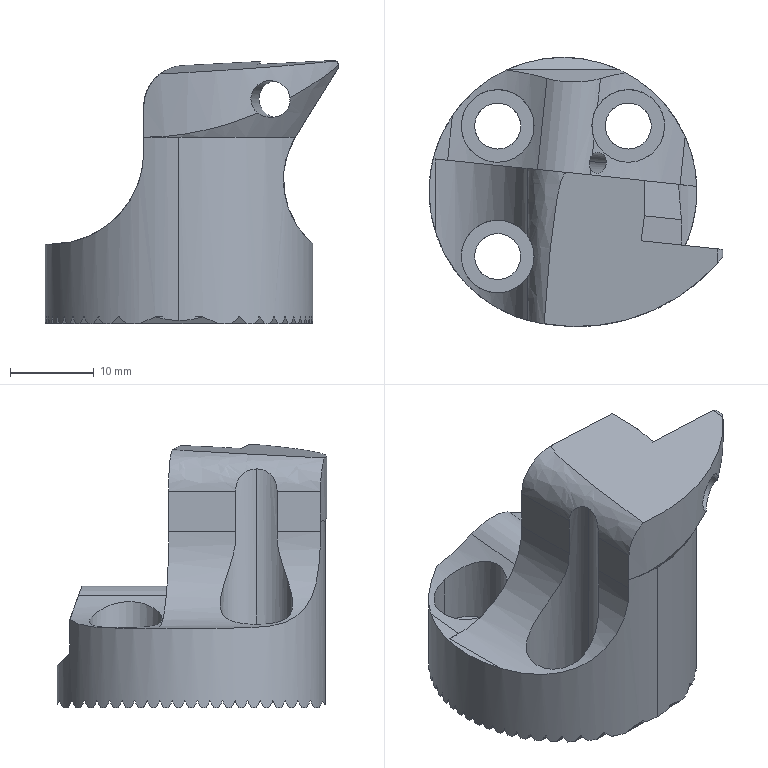NC program | Mastercam | posted with a generic post
Lines 2598 to 3368 of 7170:
(12 FEMR |TOOL - 4|DIA. OFF. - 4|LEN. - 4|TOOL DIA. - 12.)
N5254 T4 M6
N5256 G0 G54 G90 X17.229 Y24.914 C6. B-90. S3500 M3
N5258 G43 H4 Z51.893
N5260 Z3.893
N5262 G1 Z2.143 F600.
N5264 X16.532 Y23.344 Z1.992 F2500.
N5266 G3 X16.3 Y22.249 Z1.893 I2.468 J-1.095
N5268 G1 Y21.65
N5270 Y21.468
N5272 G2 X17.47 Y20.267 I-46.122 J-46.07
N5274 X19.336 Y16.759 I-6.989 J-5.969
N5276 X19.905 Y13.332 I-15.597 J-4.349
N5278 X20.038 Y8.899 I-73.7 J-4.433
N5280 X20.037 Y8.592 I-73.833
N5282 X20.046 Y4.503 I-900.155 J-4.089
N5284 G1 Y4.174
N5286 X20.047 Y3.774
N5288 X20.039 Y-14.605
N5290 G2 X18.845 Y-17.934 I-6.345 J.397
N5292 X16.3 Y-20.181 I-6.207 J4.464
N5294 G1 Y-20.58
N5296 Y-20.98
N5298 G3 X18.531 Y-23.638 Z2.143 I2.7
N5300 X19. Y-23.679 I.469 J2.658
N5302 X21.7 Y-20.98 J2.699
N5304 G1 Y21.724 F9500.
N5306 G3 X19. Y24.424 I-2.7
N5308 X18.531 Y24.383 J-2.7
N5310 X16.3 Y21.724 Z1.893 I.469 J-2.659 F2500.
N5312 G1 Y21.125
N5314 Y20.919
N5316 X17.284 Y19.65
N5318 G2 X19.073 Y15.737 I-9.523 J-6.719
N5320 X19.634 Y12.071 I-19.868 J-4.917
N5322 X19.784 Y7.07 I-83.192 J-5.001
N5324 G1 Y6.941
N5326 G2 X19.796 Y2.199 I-907.654 J-4.742
N5328 G1 Y1.72
N5330 X19.797 Y1.321
N5332 X19.795 Y-12.748
N5334 G2 X18.522 Y-16.95 I-7.96 J.117
N5336 X16.84 Y-19.048 I-9.902 J6.22
N5338 G3 X16.394 Y-19.536 I1.202 J-1.547
N5340 X16.3 Y-19.752 I1.049 J-.583
N5342 G1 X17.229 Y-19.952 Z1.956
N5344 G3 X18.002 Y-20.034 Z2.008 I.773 J3.591
N5346 X19.939 Y-19.482 Z2.143 J3.673
N5348 X21.675 Y-16.361 I-1.937 J3.121 F9500.
N5350 G1 X21.674 Y-16.279
N5352 X20.827 Y21.618
N5354 G3 X18.256 Y24.132 I-2.571 J-.058
N5356 X18.122 Y24.128 J-2.572
N5358 X17.269 Y23.934 Z2.084 I.134 J-2.568 F2500.
N5360 G1 X17.261 Y23.932
N5362 X17.25 Z2.083
N5364 X17.238 Y23.928 Z2.082
N5366 X17.229 Y23.918 Z2.081
N5368 X16.532 Y22.348 Z1.967
N5370 G3 X16.3 Y21.253 Z1.893 I2.468 J-1.095
N5372 G1 Y20.654
N5374 Y20.443
N5376 X17.166 Y19.101
N5378 G2 X18.873 Y14.755 I-12.157 J-7.283
N5380 X19.42 Y10.353 I-26.123 J-5.48
N5382 X19.541 Y4.63 I-135.074 J-5.723
N5384 X19.54 Y4.109 I-135.195
N5386 X19.544 Y2.103 I-910.907 J-3.045
N5388 G1 X19.545 Y1.702
N5390 X19.535 Y-11.68
N5392 G2 X17.933 Y-16.822 I-10.259 J.375
N5394 X16.89 Y-18.329 I-14.98 J9.258
N5396 G1 X16.588 Y-18.673
N5398 G3 X16.3 Y-19.311 I.902 J-.791
N5400 G1 X17.229 Y-19.376 Z1.954
N5402 G3 X17.585 Y-19.388 Z1.978 I.356 J5.077
N5404 X19.97 Y-18.795 Z2.143 J5.089
N5406 X22.674 Y-14.299 I-2.385 J4.496 F9500.
N5408 X22.666 Y-14.006 I-5.089
N5410 G1 X20.632 Y21.299
N5412 G3 X18.142 Y23.649 I-2.49 J-.144
N5414 G1 X18.133
N5416 G3 X17.311 Y23.507 Z2.087 I.009 J-2.494 F2500.
N5418 G1 X17.229 Y23.478 Z2.081
N5420 X16.532 Y21.908 Z1.967
N5422 G3 X16.3 Y20.813 Z1.893 I2.468 J-1.095
N5424 G1 Y20.214
N5426 Y19.992
N5428 X17.089 Y18.544
N5430 G2 X18.783 Y13.266 I-15.812 J-7.986
N5432 X19.202 Y8.649 I-36.929 J-5.677
N5434 X19.296 Y1.919 I-240.012 J-6.73
N5436 X19.294 Y.877 I-240.106
N5438 G1 X19.295 Y.477
N5440 X19.285 Y-10.465
N5442 G2 X17.583 Y-16.504 I-12.292 J.205
N5444 X16.753 Y-17.863 I-27.164 J15.656
N5446 G1 X16.532 Y-18.165
N5448 G3 X16.3 Y-18.874 I.968 J-.709
N5450 X18.531 Y-21.533 Z2.143 I2.7
N5452 X19. Y-21.574 I.469 J2.659 F9500.
N5454 X21.7 Y-18.874 J2.7
N5456 G1 Y20.384
N5458 G3 X19. Y23.084 I-2.7
N5460 X18.531 Y23.043 J-2.7
N5462 X16.3 Y20.384 Z1.893 I.469 J-2.659 F2500.
N5464 G1 Y19.785
N5466 Y19.547
N5468 X17.127 Y17.736
N5470 G2 X18.6 Y12.223 I-19.73 J-8.224
N5472 X18.979 Y6.877 I-48.873 J-6.152
N5474 X19.049 Y-1.378 I-483.854 J-8.255
N5476 X19.046 Y-3.234 I-483.924
N5478 G1 Y-3.634
N5480 G2 X19.048 Y-5.166 I-711.08 J-1.532
N5482 X19.036 Y-9.344 I-711.082
N5484 X18.313 Y-13.816 I-14.616 J.066
N5486 X16.972 Y-16.793 I-16.224 J5.518
N5488 X16.483 Y-17.666 I-12.964 J6.692
N5490 G3 X16.3 Y-18.303 I1.017 J-.637
N5492 X18.531 Y-20.962 Z2.143 I2.7
N5494 X19. Y-21.003 I.469 J2.659 F9500.
N5496 X21.7 Y-18.303 J2.7
N5498 G1 Y19.961
N5500 G3 X19. Y22.661 I-2.7
N5502 X18.531 Y22.62 J-2.7
N5504 X16.3 Y19.961 Z1.893 I.469 J-2.659 F2500.
N5506 G1 Y19.362
N5508 Y19.096
N5510 X17.124 Y16.946
N5512 G2 X18.464 Y10.714 I-24.995 J-8.633
N5514 X18.756 Y4.689 I-71.672 J-6.502
N5516 X18.799 Y-4.538 I-987.949 J-9.227
N5518 X18.796 Y-6.971 I-987.992
N5520 X18.798 Y-7.368 I-34.246 J-.397
N5522 X18.674 Y-10.292 I-34.248
N5524 X17.336 Y-15.241 I-16.027 J1.678
N5526 X16.419 Y-17.203 I-130.897 J59.975
N5528 G3 X16.3 Y-17.724 I1.081 J-.521
N5530 G1 Y-18.123
N5532 G3 X18.531 Y-20.782 Z2.143 I2.7
N5534 X19. Y-20.823 I.469 J2.659 F9500.
N5536 X21.7 Y-18.123 J2.7
N5538 G1 Y19.534
N5540 G3 X19. Y22.234 I-2.7
N5542 X18.531 Y22.193 J-2.7
N5544 X16.3 Y19.534 Z1.893 I.469 J-2.659 F2500.
N5546 G1 Y18.935
N5548 Y18.631
N5550 X17.089 Y16.163
N5552 G2 X18.261 Y9.668 I-30.966 J-8.944
N5554 X18.514 Y3.312 I-88.649 J-6.704
N5556 X18.544 Y-3.285 I-719.484 J-6.597
N5558 X18.531 Y-7.642 I-719.514
N5560 X18.071 Y-11.816 I-20.911 J.19
N5562 X16.781 Y-15.675 I-21.739 J5.125
N5564 G3 X16.387 Y-16.663 I18.044 J-7.764
N5566 X16.3 Y-17.112 I1.113 J-.449
N5568 G1 Y-17.511
N5570 G3 X18.531 Y-20.17 Z2.143 I2.7
N5572 X19. Y-20.211 I.469 J2.659 F9500.
N5574 X21.7 Y-17.511 J2.7
N5576 G1 Y19.095
N5578 G3 X19. Y21.795 I-2.7
N5580 X18.531 Y21.754 J-2.7
N5582 X16.3 Y19.095 Z1.893 I.469 J-2.659 F2500.
N5584 G1 Y18.496
N5586 G3 X16.289 Y18.32 I1.469 J-.176
N5588 X16.383 Y17.801 I1.48
N5590 X16.588 Y17.053 I143.212 J38.808
N5592 G2 X18.11 Y7.728 I-38.35 J-11.047
N5594 X18.282 Y.409 I-155.498 J-7.319
N5596 G1 Y.283
N5598 G2 X18.294 Y-3.73 I-978.009 J-4.811
N5600 X18.299 Y-4.679 I-91.297 J-.949
N5602 X18.239 Y-7.998 I-91.302
N5604 X16.904 Y-14.491 I-21.128 J.961
N5606 X16.626 Y-15.264 I-111.95 J39.698
N5608 G3 X16.352 Y-16.094 I13.718 J-4.991
N5610 X16.3 Y-16.444 I1.148 J-.35
N5612 G1 Y-16.843
N5614 G3 X18.531 Y-19.502 Z2.143 I2.7
N5616 X19. Y-19.543 I.469 J2.659 F9500.
N5618 X21.7 Y-16.843 J2.7
N5620 G1 Y18.633
N5622 G3 X19. Y21.333 I-2.7
N5624 X18.531 Y21.292 J-2.7
N5626 X16.3 Y18.633 Z1.893 I.469 J-2.659 F2500.
N5628 G1 Y18.034
N5630 G3 X16.293 Y17.854 I2.193 J-.18
N5632 X16.356 Y17.329 I2.2
N5634 X16.852 Y15.044 I137.968 J28.74
N5636 G2 X17.886 Y6.703 I-47.694 J-10.149
N5638 X18.037 Y-1.115 I-202.633 J-7.818
N5640 G1 X18.036 Y-1.503
N5642 G2 X18.044 Y-3.129 I-184.424 J-1.626
N5644 X18.005 Y-6.901 I-184.431
N5646 X16.709 Y-14.114 I-24.331 J.651
N5648 G3 X16.335 Y-15.374 I21.239 J-6.982
N5650 X16.292 Y-15.821 I2.297 J-.447
N5652 X16.3 Y-16.012 I2.34
N5654 G1 Y-16.412
N5656 G3 X18.531 Y-19.071 Z2.143 I2.7
N5658 X19. Y-19.112 I.469 J2.659 F9500.
N5660 X21.7 Y-16.412 J2.7
N5662 G1 Y18.15
N5664 G3 X19. Y20.85 I-2.7
N5666 X18.531 Y20.809 J-2.7
N5668 X16.3 Y18.15 Z1.893 I.469 J-2.659 F2500.
N5670 G1 Y17.552
N5672 G3 X16.295 Y17.352 I3.979 J-.2
N5674 X16.367 Y16.596 I3.984
N5676 X16.887 Y13.556 I127.277 J20.19
N5678 G2 X17.672 Y5.359 I-59.861 J-9.865
N5680 X17.785 Y-2.317 I-261.64 J-7.676
N5682 X17.756 Y-6.174 I-261.753
N5684 X16.655 Y-13.256 I-27.266 J.611
N5686 G3 X16.333 Y-14.475 I30.139 J-8.621
N5688 X16.291 Y-14.936 I2.485 J-.461
N5690 X16.3 Y-15.153 I2.527
N5692 G1 Y-15.552
N5694 Y-16.412
N5696 G3 X18.531 Y-19.071 Z2.143 I2.7
N5698 X19. Y-19.112 I.469 J2.659 F9500.
N5700 X21.7 Y-16.412 J2.7
N5702 G1 Y17.653
N5704 G3 X19. Y20.353 I-2.7
N5706 X18.531 Y20.312 J-2.7
N5708 X16.3 Y17.653 Z1.893 I.469 J-2.659 F2500.
N5710 G1 Y17.054
N5712 G3 X16.298 Y16.829 I10.911 J-.225
N5714 X16.434 Y15.106 I10.913
N5716 X16.76 Y12.776 I194.547 J26.008
N5718 G2 X17.453 Y3.862 I-75.233 J-10.333
N5720 X17.528 Y-2.043 I-232.58 J-5.905
N5722 X17.501 Y-5.625 I-232.655
N5724 X16.532 Y-12.578 I-30.614 J.723
N5726 G3 X16.328 Y-13.451 I39.524 J-9.682
N5728 X16.29 Y-13.882 I2.422 J-.431
N5730 X16.3 Y-14.107 I2.46
N5732 G1 Y-14.506
N5734 Y-15.304
N5736 G3 X18.531 Y-17.963 Z2.143 I2.7
N5738 X19. Y-18.004 I.469 J2.659 F9500.
N5740 X21.7 Y-15.304 J2.7
N5742 G1 Y17.07
N5744 G3 X19. Y19.77 I-2.7
N5746 X18.531 Y19.729 J-2.7
N5748 X16.3 Y17.07 Z1.893 I.469 J-2.659 F2500.
N5750 G1 Y16.471
N5752 G3 X16.293 Y15.956 I19.631 J-.515
N5754 X16.474 Y13.301 I19.638
N5756 X16.606 Y12.122 I443.354 J49.351
N5758 G2 X17.232 Y2.087 I-96.766 J-11.073
N5760 X17.274 Y-1.904 I-191.291 J-3.991
N5762 X17.25 Y-4.94 I-191.333
N5764 X16.349 Y-12.131 I-35.101 J.747
N5766 G3 X16.292 Y-12.677 I2.564 J-.546
N5768 X16.3 Y-12.893 I2.621
N5770 G1 Y-13.292
N5772 Y-14.091
N5774 G3 X18.531 Y-16.75 Z2.143 I2.7
N5776 X19. Y-16.791 I.469 J2.659 F9500.
N5778 X21.7 Y-14.091 J2.7
N5780 G1 Y16.127
N5782 G3 X19. Y18.827 I-2.7
N5784 X18.531 Y18.786 J-2.7
N5786 X16.3 Y16.127 Z1.893 I.469 J-2.659 F2500.
N5788 G1 Y16.
N5790 G3 X16.298 Y15.364 I108.844 J-.636
N5792 X16.317 Y13.347 I108.846
N5794 X16.616 Y9.542 I117.647 J7.325
N5796 G2 X17.01 Y-.388 I-136.081 J-10.375
N5798 X17.023 Y-1.91 I-88.03 J-1.522
N5800 X16.931 Y-5.925 I-88.043
N5802 X16.318 Y-10.85 I-37.817 J2.21
N5804 G3 X16.291 Y-11.234 I2.726 J-.384
N5806 X16.3 Y-11.456 I2.753
N5808 G1 Y-11.855
N5810 Y-13.052
N5812 G3 X18.531 Y-15.711 Z2.143 I2.7
N5814 X19. Y-15.752 I.469 J2.659 F9500.
N5816 X21.7 Y-13.052 J2.7
N5818 G1 Y14.531
N5820 G3 X19. Y17.231 I-2.7
N5822 X18.531 Y17.19 J-2.7
N5824 X16.3 Y14.531 Z1.893 I.469 J-2.659 F2500.
N5826 G1 Y13.932
N5828 G3 X16.296 Y13.136 I90.129 J-.796
N5830 X16.331 Y10.649 I90.133
N5832 X16.53 Y7.1 I269.457 J13.365
N5834 G2 X16.753 Y-1.507 I-166.241 J-8.607
N5836 X16.733 Y-4.089 I-166.464
N5838 X16.311 Y-9.117 I-41.747 J.97
N5840 G3 X16.292 Y-9.461 I3.141 J-.344
N5842 X16.3 Y-9.679 I3.16
N5844 G1 Y-10.078
N5846 Y-11.675
N5848 G3 X18.531 Y-14.334 Z2.143 I2.7
N5850 X19. Y-14.375 I.469 J2.659 F9500.
N5852 X21.7 Y-11.675 J2.7
N5854 G1 Y12.255
N5856 G3 X19. Y14.955 I-2.7
N5858 X18.531 Y14.914 J-2.7
N5860 X16.3 Y12.255 Z1.893 I.469 J-2.659 F2500.
N5862 G1 Y11.656
N5864 G3 X16.297 Y10.459 I266.314 J-1.197
N5866 X16.32 Y6.993 I266.317
N5868 X16.404 Y4.216 I618.068 J17.407
N5870 G2 X16.494 Y-1.161 I-161.356 J-5.377
N5872 X16.475 Y-3.654 I-161.446
N5874 X16.3 Y-6.79 I-52.915 J1.373
N5876 G1 Y-7.189
N5878 Y-9.983
N5880 G3 X18.531 Y-12.642 Z2.143 I2.7
N5882 X19. Y-12.683 I.469 J2.659 F9500.
N5884 X21.7 Y-9.983 J2.7
N5886 G1 Y8.686
N5888 G3 X19. Y11.386 I-2.7
N5890 X18.531 Y11.345 J-2.7
N5892 X16.3 Y8.686 Z1.893 I.469 J-2.659 F2500.
N5894 G1 Y8.087
N5896 Y-7.477
N5898 G3 X16.532 Y-8.573 Z1.992 I2.7
N5900 G1 X17.229 Y-10.142 Z2.143
N5902 G0 Z51.893
N5904 Z52.593
N5906 X16.2 Y24.
N5908 Z3.593
N5910 G1 Z2.593 F2000.
N5912 G41 D4 Y16. F1500.
N5914 Y-16.
N5916 G40 Y-24.
N5918 G0 Z52.593
N5920 X15.9 Y24.
N5922 Z3.593
N5924 G1 Z2.593 F2000.
N5926 G41 D4 Y16. F1500.
N5928 Y-16.
N5930 G40 Y-24.
N5932 G0 Z52.593
N5934 X15.6 Y24.
N5936 Z3.593
N5938 G1 Z2.593 F2000.
N5940 G41 D4 Y16. F1500.
N5942 Y-16.
N5944 G40 Y-24.
N5946 G0 Z52.593
N5948 Z65.5
N5950 X12.55 Y15.764
N5952 C0.
N5954 Z16.5
N5956 G1 Z15.05 F2000.
N5958 G41 D4 Y6.764 F1500.
N5960 Y-6.764
N5962 G40 Y-15.764
N5964 Z14.6 F2000.
N5966 G42 D4 Y-6.764 F1500.
N5968 Y6.764
N5970 G40 Y15.764
N5972 G0 Z65.5
N5974 X16.509 Y32.531
N5976 Z50.
N5978 Z1.
N5980 G1 Z-12. F2000.
N5982 G41 D4 Y27.531 F1000.
N5984 G3 X16.609 Y27.431 I.1
N5986 G1 X19.737
N5988 G2 X26.794 Y21.998 J-7.3
N5990 G1 X38.758 Y22.622
N5992 G2 X39.153 Y22.632 I.395 J-7.59
N5994 X46.753 Y15.032 J-7.6
N5996 X43.816 Y9.031 I-7.6
N5998 G3 X43.778 Y8.952 I.062 J-.079
N6000 X43.799 Y8.891 I.1
N6002 G1 G40 X46.866 Y4.942
N6004 G0 Z38.
N6006 X16.509 Y32.231
N6008 Z1.
N6010 G1 Z-12. F2000.
N6012 G41 D4 Y27.231 F1000.
N6014 G3 X16.609 Y27.131 I.1
N6016 G1 X19.737
N6018 G2 X26.562 Y21.686 J-7.
N6020 G1 X38.773 Y22.322
N6022 G2 X39.153 Y22.332 I.38 J-7.29
N6024 X46.453 Y15.032 J-7.3
N6026 X43.632 Y9.268 I-7.3
N6028 G3 X43.593 Y9.189 I.061 J-.079
N6030 X43.615 Y9.127 I.1
N6032 G1 G40 X46.682 Y5.179
N6034 G0 Z38.
N6036 X16.509 Y31.931
N6038 Z1.
N6040 G1 Z-12. F2000.
N6042 G41 D4 Y26.931 F1000.
N6044 G3 X16.609 Y26.831 I.1
N6046 G1 X19.737
N6048 G2 X26.321 Y21.373 J-6.7
N6050 G1 X38.789 Y22.023
N6052 G2 X39.153 Y22.032 I.364 J-6.991
N6054 X46.153 Y15.032 J-7.
N6056 X43.448 Y9.505 I-7.
N6058 G3 X43.409 Y9.426 I.061 J-.079
N6060 X43.43 Y9.364 I.1
N6062 G1 G40 X46.498 Y5.416
N6064 G0 Z38.
N6066 X16.509 Y31.631
N6068 Z1.
N6070 G1 Z-12. F2000.
N6072 G41 D4 Y26.631 F1000.
N6074 G3 X16.609 Y26.531 I.1
N6076 G1 X19.737
N6078 G2 X26.056 Y21.146 J-6.4
N6080 G3 X26.154 Y21.063 I.098 J.016
N6082 X26.18 Y21.065 J.099
N6084 G1 X38.804 Y21.723
N6086 G2 X39.153 Y21.732 I.349 J-6.691
N6088 X45.853 Y15.032 J-6.7
N6090 X43.264 Y9.742 I-6.7
N6092 G3 X43.225 Y9.663 I.061 J-.079
N6094 X43.246 Y9.601 I.1
N6096 G1 G40 X46.314 Y5.653
N6098 G0 Z38.
N6100 X16.509 Y31.331
N6102 Z1.
N6104 G1 Z-12. F2000.
N6106 G41 D4 Y26.331 F1000.
N6108 G3 X16.609 Y26.231 I.1
N6110 G1 X19.737
N6112 G2 X25.759 Y21.098 J-6.1
N6114 G3 X26.154 Y20.762 I.395 J.064
N6116 X26.215 Y20.767 J.4
N6118 G1 X38.82 Y21.424
N6120 G2 X39.153 Y21.433 I.333 J-6.392
N6122 X45.554 Y15.032 J-6.401
N6124 X43.08 Y9.978 I-6.401
N6126 G3 X43.042 Y9.9 I.061 J-.078
N6128 X43.062 Y9.838 I.099
N6130 G1 G40 X46.13 Y5.89
N6132 G0 Z50.
N6134 Z66.
N6136 X-16.529 Y-26.264
N6138 B-270.
N6140 Z18.
N6142 G1 Z-4.75 F600.
N6144 X-15.832 Y-24.694 Z-4.901 F2500.
N6146 G3 X-15.6 Y-23.599 Z-5. I-2.468 J1.095
N6148 G1 Y-23.
N6150 X-15.856 Y-22.941
N6152 G3 X-18.369 Y-22.787 I-2.632 J-22.339
N6154 X-26.489 Y-22.747 I-8.12 J-814.593
N6156 X-29.029 Y-22.75 J-814.633
N6158 G1 X-29.428
N6160 X-39.759 Y-22.745
N6162 G2 X-44.414 Y-20.758 I.082 J6.638
N6164 X-46.394 Y-17.58 I6.172 J6.052
N6166 X-47.093 Y-14.457 I12.879 J4.518
N6168 X-47.302 Y-10.354 I41.841 J4.194
N6170 X-47.329 Y-3.149 I944.127 J7.205
N6172 X-47.327 Y-1.1 I944.154
N6174 G1 Y-.701
N6176 X-47.328 Y10.048
N6178 X-48.126
N6180 G3 X-49.221 Y9.815 Z-4.925 J-2.7
N6182 G1 X-50.791 Y9.119 Z-4.811
N6184 G3 X-51.587 Y8.652 Z-4.75 I1.679 J-3.782
N6186 X-53.249 Y5.337 I2.475 J-3.315
N6188 X-53.171 Y4.533 I4.137
N6190 G1 X-48.8 Y-17.54 F9500.
N6192 G3 X-41.667 Y-24.265 I8.283 J1.64
N6194 G1 X-18.671 Y-27.428
N6196 G3 X-18.393 Y-27.447 I.278 J2.02
N6198 X-17.08 Y-26.968 J2.039
N6200 X-16.529 Y-26.235 Z-4.811 I-1.313 J1.56 F2500.
N6202 G1 X-15.832 Y-24.666 Z-4.925
N6204 G3 X-15.6 Y-23.57 Z-5. I-2.468 J1.096
N6206 G1 Y-22.971
N6208 Y-22.953
N6210 G3 X-16.317 Y-22.777 I-1.124 J-3.02
N6212 X-19.2 Y-22.558 I-3.154 J-22.437
N6214 X-25.814 Y-22.497 I-6.614 J-360.359
N6216 X-27.425 Y-22.501 J-360.42
N6218 G1 X-27.824
N6220 X-38.336 Y-22.495
N6222 G2 X-44.136 Y-19.797 I.151 J7.909
N6224 X-46.126 Y-16.277 I7.532 J6.579
N6226 X-46.832 Y-12.85 I15.165 J4.912
N6228 X-47.049 Y-8.389 I50.339 J4.685
N6230 X-47.079 Y-.727 I969.138 J7.662
N6232 X-47.077 Y1.265 I969.168
N6234 G1 Y1.664
N6236 X-47.085 Y9.063
N6238 G3 X-47.168 Y10.048 I-15.409 J-.798
N6240 G1 X-47.567
N6242 X-47.966
N6244 G3 X-49.062 Y9.815 Z-4.925 J-2.7
N6246 G1 X-50.631 Y9.119 Z-4.811
N6248 G3 X-51.428 Y8.654 Z-4.75 I1.705 J-3.84
N6250 X-53.127 Y5.279 I2.502 J-3.375 F9500.
N6252 X-52.977 Y4.164 I4.201
N6254 G1 X-46.924 Y-17.838
N6256 G3 X-39.987 Y-24.034 I8.267 J2.275
N6258 G1 X-18.72 Y-27.373
N6260 G3 X-18.402 Y-27.398 I.318 J2.024
N6262 X-17.079 Y-26.914 J2.049
N6264 X-16.529 Y-26.18 Z-4.811 I-1.323 J1.565 F2500.
N6266 G1 X-15.832 Y-24.611 Z-4.925
N6268 G3 X-15.6 Y-23.515 Z-5. I-2.468 J1.096
N6270 G1 Y-22.917
N6272 Y-22.893
N6274 G3 X-16.293 Y-22.673 I-1.241 J-2.713
N6276 X-18.987 Y-22.364 I-3.251 J-16.412
N6278 X-24.507 Y-22.255 I-5.52 J-140.011
N6280 X-25.109 Y-22.256 J-140.12
N6282 X-26.697 Y-22.253 I-2.886 J-999.355
N6284 G1 X-27.094 Y-22.252
N6286 X-36.715 Y-22.248
N6288 X-36.805
N6290 G2 X-39.816 Y-21.792 J10.146
N6292 X-44.423 Y-18.281 I2.836 J8.501
N6294 X-46.026 Y-14.712 I9.782 J6.536
N6296 X-46.629 Y-11.044 I19.657 J5.115
N6298 X-46.809 Y-5.878 I74.504 J5.186
N6300 X-46.828 Y-.045 I912.13 J5.833
N6302 X-46.827 Y.952 I912.149
N6304 G1 Y1.352
N6306 G3 X-46.825 Y3.063 I-700.542 J1.711
N6308 X-46.845 Y8.344 I-700.544
N6310 X-47.022 Y10.048 I-9.434 J-.118
N6312 G1 X-47.421
N6314 X-47.82
N6316 G3 X-48.915 Y9.815 Z-4.925 J-2.7
N6318 G1 X-50.485 Y9.119 Z-4.811
N6320 G3 X-51.281 Y8.652 Z-4.75 I1.672 J-3.767
N6322 X-52.934 Y5.352 I2.468 J-3.3 F9500.
N6324 X-52.797 Y4.299 I4.121
N6326 G1 X-47.076 Y-17.338
N6328 G3 X-40.517 Y-23.45 I8.131 J2.15
N6330 G1 X-19.19 Y-27.509
N6332 G3 X-18.738 Y-27.552 I.452 J2.375
N6334 X-17.055 Y-26.869 J2.418
N6336 X-16.529 Y-26.115 Z-4.811 I-1.683 J1.735 F2500.
N6338 G1 X-15.832 Y-24.545 Z-4.925
N6340 G3 X-15.6 Y-23.45 Z-5. I-2.468 J1.095
N6342 G1 Y-22.851
N6344 Y-22.824
N6346 G3 X-16.273 Y-22.57 I-1.338 J-2.534
N6348 X-18.827 Y-22.181 I-3.354 J-13.446
N6350 X-23.968 Y-22.018 I-5.141 J-81.004
N6352 X-24.046 Y-22.019 J-81.167
N6354 X-29.966 Y-22.001 I-5.92 J-971.018
N6356 G1 X-30.789
N6358 X-31.188
N6360 G2 X-32.317 Y-22.003 I-1.129 J346.736
N6362 X-36.19 Y-21.981 J346.738
N6364 X-39.99 Y-21.15 I.28 J10.385
N6366 X-44.321 Y-17.3 I3.986 J8.845
N6368 X-45.818 Y-13.614 I11.087 J6.65
N6370 X-46.402 Y-9.589 I23.475 J5.463
N6372 X-46.564 Y-3.879 I100.359 J5.71
N6374 G1 Y-3.674
N6376 G2 X-46.576 Y1.101 I961.751 J4.775
N6378 G1 Y1.143
N6380 Y1.543
N6382 G3 X-46.575 Y2.747 I-668.678 J1.204
N6384 X-46.592 Y7.413 I-668.679
N6386 X-46.774 Y9.557 I-13.108 J-.037
N6388 G1 X-46.882 Y10.048
N6390 X-47.68
N6392 G3 X-48.775 Y9.815 Z-4.925 J-2.7
N6394 G1 X-50.345 Y9.119 Z-4.811
N6396 G3 X-51.142 Y8.654 Z-4.75 I1.701 J-3.832
N6398 X-52.836 Y5.287 I2.498 J-3.367 F9500.
N6400 X-52.627 Y3.982 I4.192
N6402 G1 X-45.552 Y-17.606
N6404 G3 X-39.1 Y-23.331 I8.13 J2.664
N6406 G1 X-19.039 Y-27.343
N6408 G3 X-18.596 Y-27.387 I.443 J2.217
N6410 X-17.064 Y-26.789 J2.261
N6412 X-16.529 Y-26.043 Z-4.811 I-1.532 J1.663 F2500.
N6414 G1 X-15.832 Y-24.474 Z-4.925
N6416 G3 X-15.6 Y-23.378 Z-5. I-2.468 J1.096
N6418 G1 Y-22.779
N6420 Y-22.749
N6422 G3 X-16.254 Y-22.468 I-1.412 J-2.381
N6424 X-18.697 Y-22.009 I-3.441 J-11.575
N6426 X-23.419 Y-21.788 I-4.954 J-55.41
N6428 X-31.97 Y-21.746 I-8.551 J-869.741
N6430 X-34.143 Y-21.749 J-869.783
N6432 G2 X-34.406 Y-21.751 I-.263 J16.76
N6434 X-36.971 Y-21.553 J16.762
N6436 X-43.812 Y-17.032 I1.6 J9.855
N6438 X-45.404 Y-13.408 I11.023 J7.005
N6440 X-46.093 Y-9.335 I21.949 J5.807
N6442 X-46.303 Y-3.76 I75.751 J5.647
N6444 X-46.328 Y3.105 I960.668 J6.865
N6446 X-46.327 Y4.274 I960.693
N6448 G3 X-46.323 Y4.994 I-61.408 J.72
N6450 X-46.393 Y7.925 I-61.412
N6452 X-46.626 Y9.604 I-10.111 J-.549
N6454 G2 X-46.745 Y10.048 I11.621 J3.356
N6456 G1 X-47.144
N6458 X-47.543
N6460 G3 X-48.639 Y9.815 Z-4.925 J-2.7
N6462 G1 X-50.208 Y9.119 Z-4.811
N6464 G3 X-51.02 Y8.679 Z-4.75 I2.386 J-5.375
N6466 X-53.703 Y3.744 I3.198 J-4.935 F9500.
N6468 X-53.268 Y1.527 I5.881
N6470 G1 X-45.423 Y-17.734
N6472 G3 X-39.641 Y-22.725 I7.779 J3.168
N6474 G1 X-19.813 Y-27.579
N6476 G3 X-19.135 Y-27.661 I.678 J2.769
N6478 X-17.033 Y-26.737 J2.851
N6480 X-16.529 Y-25.967 Z-4.811 I-2.102 J1.927 F2500.
N6482 G1 X-15.832 Y-24.397 Z-4.925
N6484 G3 X-15.6 Y-23.302 Z-5. I-2.468 J1.095
N6486 G1 Y-22.703
N6488 Y-22.671
N6490 G3 X-16.235 Y-22.366 I-1.489 J-2.285
N6492 X-18.587 Y-21.843 I-3.528 J-10.311
N6494 X-22.828 Y-21.568 I-4.913 J-42.987
N6496 X-31.008 Y-21.497 I-8.18 J-473.743
N6498 X-32.681 Y-21.501 J-473.814
N6500 G2 X-33.044 Y-21.504 I-.363 J26.33
N6502 X-35.684 Y-21.37 J26.333
N6504 X-40.632 Y-19.53 I1.153 J10.67
N6506 X-44.193 Y-15.263 I6.353 J8.922
N6508 X-45.507 Y-11.07 I14.226 J6.76
N6510 X-45.966 Y-6.408 I34.829 J5.784
N6512 X-46.075 Y.459 I216.564 J6.867
N6514 X-46.073 Y1.383 I216.673
N6516 G1 X-46.074 Y1.784
N6518 G3 X-46.072 Y2.709 I-189.896 J.925
N6520 X-46.115 Y6.781 I-189.898
N6522 X-46.401 Y9.345 I-14.378 J-.304
N6524 X-46.611 Y10.048 I-10.426 J-2.736
N6526 G1 X-47.01
N6528 X-47.409
N6530 G3 X-48.505 Y9.815 Z-4.925 J-2.7
N6532 G1 X-50.074 Y9.119 Z-4.811
N6534 G3 X-50.872 Y8.654 Z-4.75 I1.71 J-3.853
N6536 X-52.579 Y5.266 I2.508 J-3.388 F9500.
N6538 X-52.317 Y3.801 I4.215
N6540 G1 X-44.477 Y-17.361
N6542 G3 X-42.445 Y-20.503 I8.067 J2.989
N6544 X-39.925 Y-22.127 I5.162 J5.243
N6546 G1 X-23.085 Y-28.605
N6548 G3 X-21.236 Y-28.948 I1.849 J4.807
N6550 X-16.978 Y-26.694 J5.15
N6552 X-16.529 Y-25.887 Z-4.811 I-4.258 J2.896 F2500.
N6554 G1 X-15.832 Y-24.318 Z-4.925
N6556 G3 X-15.6 Y-23.222 Z-5. I-2.468 J1.096
N6558 G1 Y-22.624
N6560 Y-22.59
N6562 G3 X-16.217 Y-22.264 I-1.499 J-2.089
N6564 X-18.489 Y-21.683 I-3.611 J-9.385
N6566 X-22.641 Y-21.347 I-5.003 J-36.011
N6568 X-30.189 Y-21.251 I-7.548 J-297.317
N6570 X-31.247 Y-21.253 J-297.413
N6572 G2 X-31.637 Y-21.255 I-.39 J43.943
N6574 X-34.473 Y-21.163 J43.945
N6576 X-38.83 Y-19.999 I.862 J11.956
N6578 X-43.408 Y-15.656 I4.948 J9.8
N6580 X-45.038 Y-11.406 I12.773 J7.338
N6582 X-45.632 Y-7.055 I27.457 J5.964
N6584 X-45.81 Y-.846 I108.379 J6.209
N6586 G1 Y-.756
N6588 G2 X-45.829 Y4.04 I897.691 J5.902
N6590 G3 X-45.828 Y4.32 I-43.747 J.28
N6592 X-45.949 Y7.576 I-43.748
N6594 X-46.302 Y9.554 I-9.818 J-.732
N6596 G1 X-46.352 Y9.694
N6598 X-46.479 Y10.048
N6600 X-47.277
N6602 G3 X-48.372 Y9.815 Z-4.925 J-2.7
N6604 G1 X-49.942 Y9.119 Z-4.811
N6606 G3 X-50.754 Y8.678 Z-4.75 I2.352 J-5.299
N6608 X-53.388 Y3.82 I3.164 J-4.858 F9500.
N6610 G1 X-53.367 Y3.332
N6612 X-53.305 Y2.848
N6614 X-53.203 Y2.371
N6616 X-53.062 Y1.904
N6618 X-52.881 Y1.45
N6620 X-44.524 Y-17.21
N6622 G3 X-39.673 Y-21.652 I7.558 J3.384
N6624 G1 X-21.465 Y-27.951
N6626 G3 X-20.164 Y-28.17 I1.301 J3.76
N6628 X-16.999 Y-26.6 J3.979
N6630 X-16.529 Y-25.805 Z-4.811 I-3.165 J2.409 F2500.
N6632 G1 X-15.832 Y-24.236 Z-4.925
N6634 G3 X-15.6 Y-23.14 Z-5. I-2.468 J1.096
N6636 G1 Y-22.542
N6638 Y-22.507
N6640 G3 X-16.199 Y-22.162 I-1.543 J-1.991
N6642 X-18.402 Y-21.528 I-3.689 J-8.668
N6644 X-22.469 Y-21.131 I-5.093 J-31.155
N6646 X-29.634 Y-21.006 I-7.165 J-205.841
N6648 X-30.233 Y-21.007 J-205.966
N6650 G2 X-30.706 Y-21.009 I-.473 J45.485
N6652 X-33.872 Y-20.899 J45.487
N6654 X-38.093 Y-19.821 I.978 J12.632
N6656 X-42.958 Y-15.43 I4.781 J10.185
N6658 X-44.673 Y-11.214 I12.641 J7.601
N6660 X-45.34 Y-6.829 I26.177 J6.222
N6662 X-45.55 Y-.894 I91.565 J6.212
N6664 X-45.585 Y4.281 I734.458 J7.641
N6666 G1 Y4.294
N6668 G3 X-45.76 Y7.704 I-33.357
N6670 X-46.166 Y9.595 I-8.908 J-.922
N6672 G2 X-46.347 Y10.048 I17.379 J7.225
N6674 G1 X-46.746
N6676 X-47.145
N6678 G3 X-48.241 Y9.815 Z-4.925 J-2.7
N6680 G1 X-49.81 Y9.119 Z-4.811
N6682 G3 X-50.606 Y8.652 Z-4.75 I1.661 J-3.743
N6684 X-52.244 Y5.376 I2.457 J-3.276 F9500.
N6686 X-51.959 Y3.875 I4.095
N6688 G1 X-43.865 Y-16.666
N6690 G3 X-38.885 Y-21.478 I7.775 J3.064
N6692 G1 X-21.233 Y-27.743
N6694 G3 X-19.973 Y-27.96 I1.26 J3.551
N6696 X-17.004 Y-26.512 J3.768
N6698 X-16.529 Y-25.721 Z-4.811 I-2.969 J2.32 F2500.
N6700 G1 X-15.832 Y-24.152 Z-4.925
N6702 G3 X-15.6 Y-23.056 Z-5. I-2.468 J1.096
N6704 G1 Y-22.457
N6706 Y-22.421
N6708 G3 X-16.182 Y-22.061 I-1.583 J-1.904
N6710 X-18.615 Y-21.319 I-4.001 J-8.77
N6712 X-22.676 Y-20.9 I-5.241 J-30.919
N6714 X-29.756 Y-20.759 I-7.08 J-177.38
N6716 G1 X-30.038
N6718 X-30.108
N6720 G2 X-33.268 Y-20.64 J41.887
N6722 X-37.353 Y-19.65 I1.071 J13.338
N6724 X-42.684 Y-14.936 I4.638 J10.615
N6726 X-44.439 Y-10.513 I13.13 J7.772
N6728 X-45.116 Y-5.722 I28.909 J6.525
N6730 X-45.305 Y.573 I108.13 J6.404
N6732 X-45.315 Y1.778 I700.13 J6.152
N6734 G1 Y2.03
N6736 G3 X-45.421 Y6.263 I-84.427
N6738 X-45.781 Y8.843 I-14.941 J-.771
N6740 X-46.217 Y10.048 I-5.567 J-1.333
N6742 G1 X-46.616
N6744 X-47.015
N6746 G3 X-48.11 Y9.815 Z-4.925 J-2.7
N6748 G1 X-49.68 Y9.119 Z-4.811
N6750 G3 X-50.492 Y8.679 Z-4.75 I2.382 J-5.365
N6752 X-53.168 Y3.754 I3.194 J-4.925 F9500.
N6754 X-52.496 Y1.029 I5.87
N6756 G1 X-42.915 Y-17.246
N6758 G3 X-38.42 Y-21.208 I7.426 J3.894
N6760 G1 X-21.243 Y-27.616
N6762 G3 X-19.939 Y-27.851 I1.304 J3.495
N6764 X-17.005 Y-26.425 J3.73
N6766 X-16.529 Y-25.635 Z-4.811 I-2.934 J2.304 F2500.
N6768 G1 X-15.832 Y-24.065 Z-4.925
N6770 G3 X-15.6 Y-22.97 Z-5. I-2.468 J1.095
N6772 G1 Y-22.371
N6774 Y-22.334
N6776 G3 X-16.164 Y-21.959 I-1.618 J-1.822
N6778 X-18.533 Y-21.166 I-4.065 J-8.213
N6780 X-22.522 Y-20.69 I-5.327 J-27.68
N6782 X-29.045 Y-20.52 I-6.709 J-132.093
N6784 G1 X-29.138
N6786 G2 X-32.662 Y-20.385 J46.101
N6788 X-36.641 Y-19.469 I1.147 J14.074
N6790 X-42.255 Y-14.717 I4.418 J10.913
N6792 X-44.086 Y-10.324 I13.085 J8.032